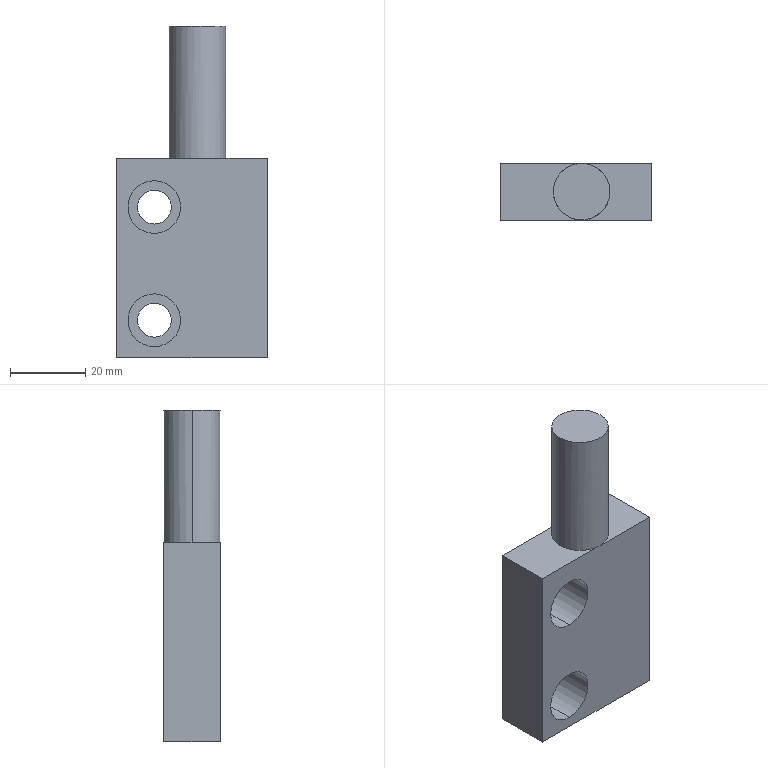Part | SolidWorks | features BaseBody 1 | 1 solid | 20 faces | box 40 x 15 x 88 mm | volume 34270 mm3 | cylinder 10 | plane 10 | commonest cylinder face diameters 9 x4 14 x4 15 x2
STEP:
#1=CARTESIAN_POINT('',(340.,-80.,242.621));
#2=VERTEX_POINT('',#1);
#3=CARTESIAN_POINT('',(340.,-80.,251.621));
#4=VERTEX_POINT('',#3);
#5=CARTESIAN_POINT('',(340.,-80.,247.121));
#6=DIRECTION('',(0.,1.,0.));
#7=DIRECTION('',(0.,0.,-1.));
#8=AXIS2_PLACEMENT_3D('',#5,#6,#7);
#9=CIRCLE('',#8,4.5);
#10=EDGE_CURVE('',#2,#4,#9,.T.);
#11=ORIENTED_EDGE('',*,*,#10,.T.);
#12=CARTESIAN_POINT('',(340.,-85.,251.621));
#13=VERTEX_POINT('',#12);
#14=CARTESIAN_POINT('',(340.,-95.,251.621));
#15=DIRECTION('',(0.,-1.,0.));
#16=VECTOR('',#15,1000.);
#17=LINE('',#14,#16);
#18=EDGE_CURVE('',#4,#13,#17,.T.);
#19=ORIENTED_EDGE('',*,*,#18,.T.);
#20=CARTESIAN_POINT('',(340.,-85.,242.621));
#21=VERTEX_POINT('',#20);
#22=CARTESIAN_POINT('',(340.,-85.,247.121));
#23=DIRECTION('',(0.,1.,0.));
#24=DIRECTION('',(0.,0.,-1.));
#25=AXIS2_PLACEMENT_3D('',#22,#23,#24);
#26=CIRCLE('',#25,4.5);
#27=EDGE_CURVE('',#21,#13,#26,.T.);
#28=ORIENTED_EDGE('',*,*,#27,.F.);
#29=CARTESIAN_POINT('',(340.,-95.,242.621));
#30=DIRECTION('',(0.,-1.,0.));
#31=VECTOR('',#30,1000.);
#32=LINE('',#29,#31);
#33=EDGE_CURVE('',#2,#21,#32,.T.);
#34=ORIENTED_EDGE('',*,*,#33,.F.);
#35=EDGE_LOOP('',(#11,#19,#28,#34));
#36=FACE_OUTER_BOUND('',#35,.T.);
#37=CARTESIAN_POINT('',(340.,-95.,247.121));
#38=DIRECTION('',(0.,-1.,0.));
#39=DIRECTION('',(0.,0.,-1.));
#40=AXIS2_PLACEMENT_3D('',#37,#38,#39);
#41=CYLINDRICAL_SURFACE('',#40,4.5);
#42=ADVANCED_FACE('',(#36),#41,.F.);
#43=CARTESIAN_POINT('',(340.,-80.,212.621));
#44=VERTEX_POINT('',#43);
#45=CARTESIAN_POINT('',(340.,-80.,221.621));
#46=VERTEX_POINT('',#45);
#47=CARTESIAN_POINT('',(340.,-80.,217.121));
#48=DIRECTION('',(0.,1.,0.));
#49=DIRECTION('',(0.,0.,-1.));
#50=AXIS2_PLACEMENT_3D('',#47,#48,#49);
#51=CIRCLE('',#50,4.5);
#52=EDGE_CURVE('',#44,#46,#51,.T.);
#53=ORIENTED_EDGE('',*,*,#52,.T.);
#54=CARTESIAN_POINT('',(340.,-85.,221.621));
#55=VERTEX_POINT('',#54);
#56=CARTESIAN_POINT('',(340.,-95.,221.621));
#57=DIRECTION('',(0.,-1.,0.));
#58=VECTOR('',#57,1000.);
#59=LINE('',#56,#58);
#60=EDGE_CURVE('',#46,#55,#59,.T.);
#61=ORIENTED_EDGE('',*,*,#60,.T.);
#62=CARTESIAN_POINT('',(340.,-85.,212.621));
#63=VERTEX_POINT('',#62);
#64=CARTESIAN_POINT('',(340.,-85.,217.121));
#65=DIRECTION('',(0.,1.,0.));
#66=DIRECTION('',(0.,0.,-1.));
#67=AXIS2_PLACEMENT_3D('',#64,#65,#66);
#68=CIRCLE('',#67,4.5);
#69=EDGE_CURVE('',#63,#55,#68,.T.);
#70=ORIENTED_EDGE('',*,*,#69,.F.);
#71=CARTESIAN_POINT('',(340.,-95.,212.621));
#72=DIRECTION('',(0.,-1.,0.));
#73=VECTOR('',#72,1000.);
#74=LINE('',#71,#73);
#75=EDGE_CURVE('',#44,#63,#74,.T.);
#76=ORIENTED_EDGE('',*,*,#75,.F.);
#77=EDGE_LOOP('',(#53,#61,#70,#76));
#78=FACE_OUTER_BOUND('',#77,.T.);
#79=CARTESIAN_POINT('',(340.,-95.,217.121));
#80=DIRECTION('',(0.,-1.,0.));
#81=DIRECTION('',(0.,0.,-1.));
#82=AXIS2_PLACEMENT_3D('',#79,#80,#81);
#83=CYLINDRICAL_SURFACE('',#82,4.5);
#84=ADVANCED_FACE('',(#78),#83,.F.);
#85=CARTESIAN_POINT('',(344.,-87.5,295.121));
#86=VERTEX_POINT('',#85);
#87=CARTESIAN_POINT('',(359.,-87.5,295.121));
#88=VERTEX_POINT('',#87);
#89=CARTESIAN_POINT('',(351.5,-87.5,295.121));
#90=DIRECTION('',(0.,0.,-1.));
#91=DIRECTION('',(-1.,0.,0.));
#92=AXIS2_PLACEMENT_3D('',#89,#90,#91);
#93=CIRCLE('',#92,7.5);
#94=EDGE_CURVE('',#86,#88,#93,.T.);
#95=ORIENTED_EDGE('',*,*,#94,.T.);
#96=CARTESIAN_POINT('',(359.,-87.5,260.121));
#97=VERTEX_POINT('',#96);
#98=CARTESIAN_POINT('',(359.,-87.5,295.121));
#99=DIRECTION('',(0.,0.,-1.));
#100=VECTOR('',#99,1000.);
#101=LINE('',#98,#100);
#102=EDGE_CURVE('',#88,#97,#101,.T.);
#103=ORIENTED_EDGE('',*,*,#102,.T.);
#104=CARTESIAN_POINT('',(351.5,-80.,260.121));
#105=VERTEX_POINT('',#104);
#106=CARTESIAN_POINT('',(351.5,-87.5,260.121));
#107=DIRECTION('',(0.,0.,1.));
#108=DIRECTION('',(-1.,0.,0.));
#109=AXIS2_PLACEMENT_3D('',#106,#107,#108);
#110=CIRCLE('',#109,7.5);
#111=EDGE_CURVE('',#97,#105,#110,.T.);
#112=ORIENTED_EDGE('',*,*,#111,.T.);
#113=CARTESIAN_POINT('',(344.,-87.5,260.121));
#114=VERTEX_POINT('',#113);
#115=CARTESIAN_POINT('',(351.5,-87.5,260.121));
#116=DIRECTION('',(0.,0.,1.));
#117=DIRECTION('',(-1.,0.,0.));
#118=AXIS2_PLACEMENT_3D('',#115,#116,#117);
#119=CIRCLE('',#118,7.5);
#120=EDGE_CURVE('',#105,#114,#119,.T.);
#121=ORIENTED_EDGE('',*,*,#120,.T.);
#122=CARTESIAN_POINT('',(344.,-87.5,295.121));
#123=DIRECTION('',(0.,0.,-1.));
#124=VECTOR('',#123,1000.);
#125=LINE('',#122,#124);
#126=EDGE_CURVE('',#86,#114,#125,.T.);
#127=ORIENTED_EDGE('',*,*,#126,.F.);
#128=EDGE_LOOP('',(#95,#103,#112,#121,#127));
#129=FACE_OUTER_BOUND('',#128,.T.);
#130=CARTESIAN_POINT('',(351.5,-87.5,295.121));
#131=DIRECTION('',(0.,0.,-1.));
#132=DIRECTION('',(-1.,0.,0.));
#133=AXIS2_PLACEMENT_3D('',#130,#131,#132);
#134=CYLINDRICAL_SURFACE('',#133,7.5);
#135=ADVANCED_FACE('',(#129),#134,.T.);
#136=CARTESIAN_POINT('',(340.,-85.,254.121));
#137=VERTEX_POINT('',#136);
#138=CARTESIAN_POINT('',(340.,-85.,240.121));
#139=VERTEX_POINT('',#138);
#140=CARTESIAN_POINT('',(340.,-85.,247.121));
#141=DIRECTION('',(0.,-1.,0.));
#142=DIRECTION('',(0.,0.,-1.));
#143=AXIS2_PLACEMENT_3D('',#140,#141,#142);
#144=CIRCLE('',#143,7.);
#145=EDGE_CURVE('',#137,#139,#144,.T.);
#146=ORIENTED_EDGE('',*,*,#145,.F.);
#147=CARTESIAN_POINT('',(340.,-95.,254.121));
#148=VERTEX_POINT('',#147);
#149=CARTESIAN_POINT('',(340.,-85.,254.121));
#150=DIRECTION('',(0.,-1.,0.));
#151=VECTOR('',#150,1000.);
#152=LINE('',#149,#151);
#153=EDGE_CURVE('',#137,#148,#152,.T.);
#154=ORIENTED_EDGE('',*,*,#153,.T.);
#155=CARTESIAN_POINT('',(340.,-95.,240.121));
#156=VERTEX_POINT('',#155);
#157=CARTESIAN_POINT('',(340.,-95.,247.121));
#158=DIRECTION('',(0.,-1.,0.));
#159=DIRECTION('',(0.,0.,-1.));
#160=AXIS2_PLACEMENT_3D('',#157,#158,#159);
#161=CIRCLE('',#160,7.);
#162=EDGE_CURVE('',#148,#156,#161,.T.);
#163=ORIENTED_EDGE('',*,*,#162,.T.);
#164=CARTESIAN_POINT('',(340.,-85.,240.121));
#165=DIRECTION('',(0.,-1.,0.));
#166=VECTOR('',#165,1000.);
#167=LINE('',#164,#166);
#168=EDGE_CURVE('',#139,#156,#167,.T.);
#169=ORIENTED_EDGE('',*,*,#168,.F.);
#170=EDGE_LOOP('',(#146,#154,#163,#169));
#171=FACE_OUTER_BOUND('',#170,.T.);
#172=CARTESIAN_POINT('',(340.,-85.,247.121));
#173=DIRECTION('',(0.,-1.,0.));
#174=DIRECTION('',(0.,0.,-1.));
#175=AXIS2_PLACEMENT_3D('',#172,#173,#174);
#176=CYLINDRICAL_SURFACE('',#175,7.);
#177=ADVANCED_FACE('',(#171),#176,.F.);
#178=CARTESIAN_POINT('',(340.,-85.,224.121));
#179=VERTEX_POINT('',#178);
#180=CARTESIAN_POINT('',(340.,-85.,210.121));
#181=VERTEX_POINT('',#180);
#182=CARTESIAN_POINT('',(340.,-85.,217.121));
#183=DIRECTION('',(0.,-1.,0.));
#184=DIRECTION('',(0.,0.,-1.));
#185=AXIS2_PLACEMENT_3D('',#182,#183,#184);
#186=CIRCLE('',#185,7.);
#187=EDGE_CURVE('',#179,#181,#186,.T.);
#188=ORIENTED_EDGE('',*,*,#187,.F.);
#189=CARTESIAN_POINT('',(340.,-95.,224.121));
#190=VERTEX_POINT('',#189);
#191=CARTESIAN_POINT('',(340.,-85.,224.121));
#192=DIRECTION('',(0.,-1.,0.));
#193=VECTOR('',#192,1000.);
#194=LINE('',#191,#193);
#195=EDGE_CURVE('',#179,#190,#194,.T.);
#196=ORIENTED_EDGE('',*,*,#195,.T.);
#197=CARTESIAN_POINT('',(340.,-95.,210.121));
#198=VERTEX_POINT('',#197);
#199=CARTESIAN_POINT('',(340.,-95.,217.121));
#200=DIRECTION('',(0.,-1.,0.));
#201=DIRECTION('',(0.,0.,-1.));
#202=AXIS2_PLACEMENT_3D('',#199,#200,#201);
#203=CIRCLE('',#202,7.);
#204=EDGE_CURVE('',#190,#198,#203,.T.);
#205=ORIENTED_EDGE('',*,*,#204,.T.);
#206=CARTESIAN_POINT('',(340.,-85.,210.121));
#207=DIRECTION('',(0.,-1.,0.));
#208=VECTOR('',#207,1000.);
#209=LINE('',#206,#208);
#210=EDGE_CURVE('',#181,#198,#209,.T.);
#211=ORIENTED_EDGE('',*,*,#210,.F.);
#212=EDGE_LOOP('',(#188,#196,#205,#211));
#213=FACE_OUTER_BOUND('',#212,.T.);
#214=CARTESIAN_POINT('',(340.,-85.,217.121));
#215=DIRECTION('',(0.,-1.,0.));
#216=DIRECTION('',(0.,0.,-1.));
#217=AXIS2_PLACEMENT_3D('',#214,#215,#216);
#218=CYLINDRICAL_SURFACE('',#217,7.);
#219=ADVANCED_FACE('',(#213),#218,.F.);
#220=CARTESIAN_POINT('',(370.,-80.,260.121));
#221=VERTEX_POINT('',#220);
#222=CARTESIAN_POINT('',(330.,-80.,260.121));
#223=DIRECTION('',(-1.,0.,0.));
#224=VECTOR('',#223,1000.);
#225=LINE('',#222,#224);
#226=EDGE_CURVE('',#221,#105,#225,.T.);
#227=ORIENTED_EDGE('',*,*,#226,.F.);
#228=CARTESIAN_POINT('',(370.,-80.,207.121));
#229=VERTEX_POINT('',#228);
#230=CARTESIAN_POINT('',(370.,-80.,260.121));
#231=DIRECTION('',(0.,0.,1.));
#232=VECTOR('',#231,1000.);
#233=LINE('',#230,#232);
#234=EDGE_CURVE('',#229,#221,#233,.T.);
#235=ORIENTED_EDGE('',*,*,#234,.F.);
#236=CARTESIAN_POINT('',(330.,-80.,207.121));
#237=VERTEX_POINT('',#236);
#238=CARTESIAN_POINT('',(330.,-80.,207.121));
#239=DIRECTION('',(1.,0.,0.));
#240=VECTOR('',#239,1000.);
#241=LINE('',#238,#240);
#242=EDGE_CURVE('',#237,#229,#241,.T.);
#243=ORIENTED_EDGE('',*,*,#242,.F.);
#244=CARTESIAN_POINT('',(330.,-80.,260.121));
#245=VERTEX_POINT('',#244);
#246=CARTESIAN_POINT('',(330.,-80.,260.121));
#247=DIRECTION('',(0.,0.,-1.));
#248=VECTOR('',#247,1000.);
#249=LINE('',#246,#248);
#250=EDGE_CURVE('',#245,#237,#249,.T.);
#251=ORIENTED_EDGE('',*,*,#250,.F.);
#252=CARTESIAN_POINT('',(330.,-80.,260.121));
#253=DIRECTION('',(-1.,0.,0.));
#254=VECTOR('',#253,1000.);
#255=LINE('',#252,#254);
#256=EDGE_CURVE('',#105,#245,#255,.T.);
#257=ORIENTED_EDGE('',*,*,#256,.F.);
#258=EDGE_LOOP('',(#227,#235,#243,#251,#257));
#259=FACE_OUTER_BOUND('',#258,.T.);
#260=ORIENTED_EDGE('',*,*,#10,.F.);
#261=CARTESIAN_POINT('',(340.,-80.,247.121));
#262=DIRECTION('',(0.,1.,0.));
#263=DIRECTION('',(0.,0.,-1.));
#264=AXIS2_PLACEMENT_3D('',#261,#262,#263);
#265=CIRCLE('',#264,4.5);
#266=EDGE_CURVE('',#4,#2,#265,.T.);
#267=ORIENTED_EDGE('',*,*,#266,.F.);
#268=EDGE_LOOP('',(#260,#267));
#269=FACE_BOUND('',#268,.T.);
#270=ORIENTED_EDGE('',*,*,#52,.F.);
#271=CARTESIAN_POINT('',(340.,-80.,217.121));
#272=DIRECTION('',(0.,1.,0.));
#273=DIRECTION('',(0.,0.,-1.));
#274=AXIS2_PLACEMENT_3D('',#271,#272,#273);
#275=CIRCLE('',#274,4.5);
#276=EDGE_CURVE('',#46,#44,#275,.T.);
#277=ORIENTED_EDGE('',*,*,#276,.F.);
#278=EDGE_LOOP('',(#270,#277));
#279=FACE_BOUND('',#278,.T.);
#280=CARTESIAN_POINT('',(330.,-80.,260.121));
#281=DIRECTION('',(0.,-1.,0.));
#282=DIRECTION('',(0.,0.,-1.));
#283=AXIS2_PLACEMENT_3D('',#280,#281,#282);
#284=PLANE('',#283);
#285=ADVANCED_FACE('',(#259,#269,#279),#284,.F.);
#286=ORIENTED_EDGE('',*,*,#120,.F.);
#287=ORIENTED_EDGE('',*,*,#256,.T.);
#288=CARTESIAN_POINT('',(330.,-95.,260.121));
#289=VERTEX_POINT('',#288);
#290=CARTESIAN_POINT('',(330.,-95.,260.121));
#291=DIRECTION('',(0.,1.,0.));
#292=VECTOR('',#291,1000.);
#293=LINE('',#290,#292);
#294=EDGE_CURVE('',#289,#245,#293,.T.);
#295=ORIENTED_EDGE('',*,*,#294,.F.);
#296=CARTESIAN_POINT('',(351.5,-95.,260.121));
#297=VERTEX_POINT('',#296);
#298=CARTESIAN_POINT('',(330.,-95.,260.121));
#299=DIRECTION('',(-1.,0.,0.));
#300=VECTOR('',#299,1000.);
#301=LINE('',#298,#300);
#302=EDGE_CURVE('',#297,#289,#301,.T.);
#303=ORIENTED_EDGE('',*,*,#302,.F.);
#304=CARTESIAN_POINT('',(351.5,-87.5,260.121));
#305=DIRECTION('',(0.,0.,1.));
#306=DIRECTION('',(-1.,0.,0.));
#307=AXIS2_PLACEMENT_3D('',#304,#305,#306);
#308=CIRCLE('',#307,7.5);
#309=EDGE_CURVE('',#114,#297,#308,.T.);
#310=ORIENTED_EDGE('',*,*,#309,.F.);
#311=EDGE_LOOP('',(#286,#287,#295,#303,#310));
#312=FACE_OUTER_BOUND('',#311,.T.);
#313=CARTESIAN_POINT('',(330.,-95.,260.121));
#314=DIRECTION('',(0.,0.,-1.));
#315=DIRECTION('',(-1.,0.,0.));
#316=AXIS2_PLACEMENT_3D('',#313,#314,#315);
#317=PLANE('',#316);
#318=ADVANCED_FACE('',(#312),#317,.F.);
#319=CARTESIAN_POINT('',(351.5,-87.5,260.121));
#320=DIRECTION('',(0.,0.,1.));
#321=DIRECTION('',(-1.,0.,0.));
#322=AXIS2_PLACEMENT_3D('',#319,#320,#321);
#323=CIRCLE('',#322,7.5);
#324=EDGE_CURVE('',#297,#97,#323,.T.);
#325=ORIENTED_EDGE('',*,*,#324,.F.);
#326=CARTESIAN_POINT('',(370.,-95.,260.121));
#327=VERTEX_POINT('',#326);
#328=CARTESIAN_POINT('',(330.,-95.,260.121));
#329=DIRECTION('',(-1.,0.,0.));
#330=VECTOR('',#329,1000.);
#331=LINE('',#328,#330);
#332=EDGE_CURVE('',#327,#297,#331,.T.);
#333=ORIENTED_EDGE('',*,*,#332,.F.);
#334=CARTESIAN_POINT('',(370.,-95.,260.121));
#335=DIRECTION('',(0.,-1.,0.));
#336=VECTOR('',#335,1000.);
#337=LINE('',#334,#336);
#338=EDGE_CURVE('',#221,#327,#337,.T.);
#339=ORIENTED_EDGE('',*,*,#338,.F.);
#340=ORIENTED_EDGE('',*,*,#226,.T.);
#341=ORIENTED_EDGE('',*,*,#111,.F.);
#342=EDGE_LOOP('',(#325,#333,#339,#340,#341));
#343=FACE_OUTER_BOUND('',#342,.T.);
#344=CARTESIAN_POINT('',(330.,-95.,260.121));
#345=DIRECTION('',(0.,0.,-1.));
#346=DIRECTION('',(-1.,0.,0.));
#347=AXIS2_PLACEMENT_3D('',#344,#345,#346);
#348=PLANE('',#347);
#349=ADVANCED_FACE('',(#343),#348,.F.);
#350=ORIENTED_EDGE('',*,*,#234,.T.);
#351=ORIENTED_EDGE('',*,*,#338,.T.);
#352=CARTESIAN_POINT('',(370.,-95.,207.121));
#353=VERTEX_POINT('',#352);
#354=CARTESIAN_POINT('',(370.,-95.,233.621));
#355=DIRECTION('',(0.,0.,-1.));
#356=VECTOR('',#355,1000.);
#357=LINE('',#354,#356);
#358=EDGE_CURVE('',#327,#353,#357,.T.);
#359=ORIENTED_EDGE('',*,*,#358,.T.);
#360=CARTESIAN_POINT('',(370.,-87.5,207.121));
#361=DIRECTION('',(0.,1.,0.));
#362=VECTOR('',#361,1000.);
#363=LINE('',#360,#362);
#364=EDGE_CURVE('',#353,#229,#363,.T.);
#365=ORIENTED_EDGE('',*,*,#364,.T.);
#366=EDGE_LOOP('',(#350,#351,#359,#365));
#367=FACE_OUTER_BOUND('',#366,.T.);
#368=CARTESIAN_POINT('',(370.,-87.5,233.621));
#369=DIRECTION('',(1.,0.,0.));
#370=DIRECTION('',(0.,0.,-1.));
#371=AXIS2_PLACEMENT_3D('',#368,#369,#370);
#372=PLANE('',#371);
#373=ADVANCED_FACE('',(#367),#372,.T.);
#374=ORIENTED_EDGE('',*,*,#364,.F.);
#375=CARTESIAN_POINT('',(330.,-95.,207.121));
#376=VERTEX_POINT('',#375);
#377=CARTESIAN_POINT('',(330.,-95.,207.121));
#378=DIRECTION('',(1.,0.,0.));
#379=VECTOR('',#378,1000.);
#380=LINE('',#377,#379);
#381=EDGE_CURVE('',#376,#353,#380,.T.);
#382=ORIENTED_EDGE('',*,*,#381,.F.);
#383=CARTESIAN_POINT('',(330.,-95.,207.121));
#384=DIRECTION('',(0.,-1.,0.));
#385=VECTOR('',#384,1000.);
#386=LINE('',#383,#385);
#387=EDGE_CURVE('',#237,#376,#386,.T.);
#388=ORIENTED_EDGE('',*,*,#387,.F.);
#389=ORIENTED_EDGE('',*,*,#242,.T.);
#390=EDGE_LOOP('',(#374,#382,#388,#389));
#391=FACE_OUTER_BOUND('',#390,.T.);
#392=CARTESIAN_POINT('',(330.,-95.,207.121));
#393=DIRECTION('',(0.,0.,1.));
#394=DIRECTION('',(1.,0.,0.));
#395=AXIS2_PLACEMENT_3D('',#392,#393,#394);
#396=PLANE('',#395);
#397=ADVANCED_FACE('',(#391),#396,.F.);
#398=ORIENTED_EDGE('',*,*,#294,.T.);
#399=ORIENTED_EDGE('',*,*,#250,.T.);
#400=ORIENTED_EDGE('',*,*,#387,.T.);
#401=CARTESIAN_POINT('',(330.,-95.,233.621));
#402=DIRECTION('',(0.,0.,1.));
#403=VECTOR('',#402,1000.);
#404=LINE('',#401,#403);
#405=EDGE_CURVE('',#376,#289,#404,.T.);
#406=ORIENTED_EDGE('',*,*,#405,.T.);
#407=EDGE_LOOP('',(#398,#399,#400,#406));
#408=FACE_OUTER_BOUND('',#407,.T.);
#409=CARTESIAN_POINT('',(330.,-87.5,233.621));
#410=DIRECTION('',(-1.,0.,0.));
#411=DIRECTION('',(0.,0.,1.));
#412=AXIS2_PLACEMENT_3D('',#409,#410,#411);
#413=PLANE('',#412);
#414=ADVANCED_FACE('',(#408),#413,.T.);
#415=ORIENTED_EDGE('',*,*,#18,.F.);
#416=ORIENTED_EDGE('',*,*,#266,.T.);
#417=ORIENTED_EDGE('',*,*,#33,.T.);
#418=CARTESIAN_POINT('',(340.,-85.,247.121));
#419=DIRECTION('',(0.,1.,0.));
#420=DIRECTION('',(0.,0.,-1.));
#421=AXIS2_PLACEMENT_3D('',#418,#419,#420);
#422=CIRCLE('',#421,4.5);
#423=EDGE_CURVE('',#13,#21,#422,.T.);
#424=ORIENTED_EDGE('',*,*,#423,.F.);
#425=EDGE_LOOP('',(#415,#416,#417,#424));
#426=FACE_OUTER_BOUND('',#425,.T.);
#427=CARTESIAN_POINT('',(340.,-95.,247.121));
#428=DIRECTION('',(0.,-1.,0.));
#429=DIRECTION('',(0.,0.,-1.));
#430=AXIS2_PLACEMENT_3D('',#427,#428,#429);
#431=CYLINDRICAL_SURFACE('',#430,4.5);
#432=ADVANCED_FACE('',(#426),#431,.F.);
#433=ORIENTED_EDGE('',*,*,#60,.F.);
#434=ORIENTED_EDGE('',*,*,#276,.T.);
#435=ORIENTED_EDGE('',*,*,#75,.T.);
#436=CARTESIAN_POINT('',(340.,-85.,217.121));
#437=DIRECTION('',(0.,1.,0.));
#438=DIRECTION('',(0.,0.,-1.));
#439=AXIS2_PLACEMENT_3D('',#436,#437,#438);
#440=CIRCLE('',#439,4.5);
#441=EDGE_CURVE('',#55,#63,#440,.T.);
#442=ORIENTED_EDGE('',*,*,#441,.F.);
#443=EDGE_LOOP('',(#433,#434,#435,#442));
#444=FACE_OUTER_BOUND('',#443,.T.);
#445=CARTESIAN_POINT('',(340.,-95.,217.121));
#446=DIRECTION('',(0.,-1.,0.));
#447=DIRECTION('',(0.,0.,-1.));
#448=AXIS2_PLACEMENT_3D('',#445,#446,#447);
#449=CYLINDRICAL_SURFACE('',#448,4.5);
#450=ADVANCED_FACE('',(#444),#449,.F.);
#451=ORIENTED_EDGE('',*,*,#102,.F.);
#452=CARTESIAN_POINT('',(351.5,-87.5,295.121));
#453=DIRECTION('',(0.,0.,-1.));
#454=DIRECTION('',(-1.,0.,0.));
#455=AXIS2_PLACEMENT_3D('',#452,#453,#454);
#456=CIRCLE('',#455,7.5);
#457=EDGE_CURVE('',#88,#86,#456,.T.);
#458=ORIENTED_EDGE('',*,*,#457,.T.);
#459=ORIENTED_EDGE('',*,*,#126,.T.);
#460=ORIENTED_EDGE('',*,*,#309,.T.);
#461=ORIENTED_EDGE('',*,*,#324,.T.);
#462=EDGE_LOOP('',(#451,#458,#459,#460,#461));
#463=FACE_OUTER_BOUND('',#462,.T.);
#464=CARTESIAN_POINT('',(351.5,-87.5,295.121));
#465=DIRECTION('',(0.,0.,-1.));
#466=DIRECTION('',(-1.,0.,0.));
#467=AXIS2_PLACEMENT_3D('',#464,#465,#466);
#468=CYLINDRICAL_SURFACE('',#467,7.5);
#469=ADVANCED_FACE('',(#463),#468,.T.);
#470=ORIENTED_EDGE('',*,*,#358,.F.);
#471=ORIENTED_EDGE('',*,*,#332,.T.);
#472=ORIENTED_EDGE('',*,*,#302,.T.);
#473=ORIENTED_EDGE('',*,*,#405,.F.);
#474=ORIENTED_EDGE('',*,*,#381,.T.);
#475=EDGE_LOOP('',(#470,#471,#472,#473,#474));
#476=FACE_OUTER_BOUND('',#475,.T.);
#477=CARTESIAN_POINT('',(340.,-95.,247.121));
#478=DIRECTION('',(0.,-1.,0.));
#479=DIRECTION('',(0.,0.,-1.));
#480=AXIS2_PLACEMENT_3D('',#477,#478,#479);
#481=CIRCLE('',#480,7.);
#482=EDGE_CURVE('',#156,#148,#481,.T.);
#483=ORIENTED_EDGE('',*,*,#482,.F.);
#484=ORIENTED_EDGE('',*,*,#162,.F.);
#485=EDGE_LOOP('',(#483,#484));
#486=FACE_BOUND('',#485,.T.);
#487=CARTESIAN_POINT('',(340.,-95.,217.121));
#488=DIRECTION('',(0.,-1.,0.));
#489=DIRECTION('',(0.,0.,-1.));
#490=AXIS2_PLACEMENT_3D('',#487,#488,#489);
#491=CIRCLE('',#490,7.);
#492=EDGE_CURVE('',#198,#190,#491,.T.);
#493=ORIENTED_EDGE('',*,*,#492,.F.);
#494=ORIENTED_EDGE('',*,*,#204,.F.);
#495=EDGE_LOOP('',(#493,#494));
#496=FACE_BOUND('',#495,.T.);
#497=CARTESIAN_POINT('',(330.,-95.,260.121));
#498=DIRECTION('',(0.,1.,0.));
#499=DIRECTION('',(0.,0.,1.));
#500=AXIS2_PLACEMENT_3D('',#497,#498,#499);
#501=PLANE('',#500);
#502=ADVANCED_FACE('',(#476,#486,#496),#501,.F.);
#503=ORIENTED_EDGE('',*,*,#27,.T.);
#504=ORIENTED_EDGE('',*,*,#423,.T.);
#505=EDGE_LOOP('',(#503,#504));
#506=FACE_BOUND('',#505,.T.);
#507=CARTESIAN_POINT('',(340.,-85.,247.121));
#508=DIRECTION('',(0.,-1.,0.));
#509=DIRECTION('',(0.,0.,-1.));
#510=AXIS2_PLACEMENT_3D('',#507,#508,#509);
#511=CIRCLE('',#510,7.);
#512=EDGE_CURVE('',#139,#137,#511,.T.);
#513=ORIENTED_EDGE('',*,*,#512,.T.);
#514=ORIENTED_EDGE('',*,*,#145,.T.);
#515=EDGE_LOOP('',(#513,#514));
#516=FACE_OUTER_BOUND('',#515,.T.);
#517=CARTESIAN_POINT('',(340.,-85.,247.121));
#518=DIRECTION('',(0.,-1.,0.));
#519=DIRECTION('',(0.,0.,-1.));
#520=AXIS2_PLACEMENT_3D('',#517,#518,#519);
#521=PLANE('',#520);
#522=ADVANCED_FACE('',(#506,#516),#521,.T.);
#523=ORIENTED_EDGE('',*,*,#69,.T.);
#524=ORIENTED_EDGE('',*,*,#441,.T.);
#525=EDGE_LOOP('',(#523,#524));
#526=FACE_BOUND('',#525,.T.);
#527=CARTESIAN_POINT('',(340.,-85.,217.121));
#528=DIRECTION('',(0.,-1.,0.));
#529=DIRECTION('',(0.,0.,-1.));
#530=AXIS2_PLACEMENT_3D('',#527,#528,#529);
#531=CIRCLE('',#530,7.);
#532=EDGE_CURVE('',#181,#179,#531,.T.);
#533=ORIENTED_EDGE('',*,*,#532,.T.);
#534=ORIENTED_EDGE('',*,*,#187,.T.);
#535=EDGE_LOOP('',(#533,#534));
#536=FACE_OUTER_BOUND('',#535,.T.);
#537=CARTESIAN_POINT('',(340.,-85.,217.121));
#538=DIRECTION('',(0.,-1.,0.));
#539=DIRECTION('',(0.,0.,-1.));
#540=AXIS2_PLACEMENT_3D('',#537,#538,#539);
#541=PLANE('',#540);
#542=ADVANCED_FACE('',(#526,#536),#541,.T.);
#543=ORIENTED_EDGE('',*,*,#94,.F.);
#544=ORIENTED_EDGE('',*,*,#457,.F.);
#545=EDGE_LOOP('',(#543,#544));
#546=FACE_OUTER_BOUND('',#545,.T.);
#547=CARTESIAN_POINT('',(351.5,-87.5,295.121));
#548=DIRECTION('',(0.,0.,1.));
#549=DIRECTION('',(1.,0.,0.));
#550=AXIS2_PLACEMENT_3D('',#547,#548,#549);
#551=PLANE('',#550);
#552=ADVANCED_FACE('',(#546),#551,.T.);
#553=ORIENTED_EDGE('',*,*,#153,.F.);
#554=ORIENTED_EDGE('',*,*,#512,.F.);
#555=ORIENTED_EDGE('',*,*,#168,.T.);
#556=ORIENTED_EDGE('',*,*,#482,.T.);
#557=EDGE_LOOP('',(#553,#554,#555,#556));
#558=FACE_OUTER_BOUND('',#557,.T.);
#559=CARTESIAN_POINT('',(340.,-85.,247.121));
#560=DIRECTION('',(0.,-1.,0.));
#561=DIRECTION('',(0.,0.,-1.));
#562=AXIS2_PLACEMENT_3D('',#559,#560,#561);
#563=CYLINDRICAL_SURFACE('',#562,7.);
#564=ADVANCED_FACE('',(#558),#563,.F.);
#565=ORIENTED_EDGE('',*,*,#195,.F.);
#566=ORIENTED_EDGE('',*,*,#532,.F.);
#567=ORIENTED_EDGE('',*,*,#210,.T.);
#568=ORIENTED_EDGE('',*,*,#492,.T.);
#569=EDGE_LOOP('',(#565,#566,#567,#568));
#570=FACE_OUTER_BOUND('',#569,.T.);
#571=CARTESIAN_POINT('',(340.,-85.,217.121));
#572=DIRECTION('',(0.,-1.,0.));
#573=DIRECTION('',(0.,0.,-1.));
#574=AXIS2_PLACEMENT_3D('',#571,#572,#573);
#575=CYLINDRICAL_SURFACE('',#574,7.);
#576=ADVANCED_FACE('',(#570),#575,.F.);
#577=CLOSED_SHELL('',(#42,#84,#135,#177,#219,#285,#318,#349,#373,#397,#414,#432,#450,#469,#502,#522,#542,#552,#564,#576));
#578=MANIFOLD_SOLID_BREP('',#577);
#579=CARTESIAN_POINT('',(0.,0.,0.));
#580=DIRECTION('',(0.,0.,1.));
#581=DIRECTION('',(1.,0.,0.));
#582=AXIS2_PLACEMENT_3D('',#579,#580,#581);
#583=(LENGTH_UNIT()NAMED_UNIT(*)SI_UNIT(.MILLI.,.METRE.));
#584=UNCERTAINTY_MEASURE_WITH_UNIT(LENGTH_MEASURE(0.00001),#583,'','');
#585=(NAMED_UNIT(*)PLANE_ANGLE_UNIT()SI_UNIT($,.RADIAN.));
#586=(NAMED_UNIT(*)SI_UNIT($,.STERADIAN.)SOLID_ANGLE_UNIT());
#587=(GEOMETRIC_REPRESENTATION_CONTEXT(3)GLOBAL_UNCERTAINTY_ASSIGNED_CONTEXT((#584))GLOBAL_UNIT_ASSIGNED_CONTEXT((#583,#585,#586))REPRESENTATION_CONTEXT('',''));
#588=ADVANCED_BREP_SHAPE_REPRESENTATION('',(#578,#582),#587);